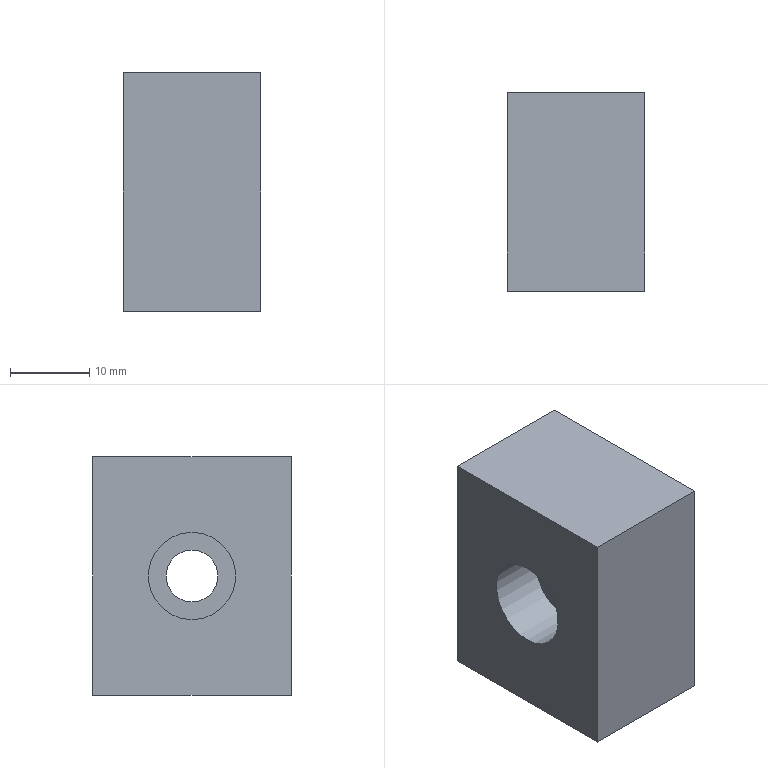Part | STEP file | SPACE-OLATE-INSERT_id702_x_t | 1 solid | 9 faces | box 17.329 x 25 x 30 mm | volume 11989 mm3 | plane 7 | cylinder 2 | commonest cylinder face diameters 6.5 x1 11 x1
STEP:
#1=CARTESIAN_POINT('',(121.671,-163.,93.));
#2=VERTEX_POINT('',#1);
#3=CARTESIAN_POINT('',(121.671,-163.,87.5));
#4=DIRECTION('',(-1.,0.,0.));
#5=DIRECTION('',(0.,0.,1.));
#6=AXIS2_PLACEMENT_3D('',#3,#4,#5);
#7=CIRCLE('',#6,5.5);
#8=EDGE_CURVE('',#2,#2,#7,.T.);
#9=ORIENTED_EDGE('',*,*,#8,.F.);
#10=EDGE_LOOP('',(#9));
#11=FACE_BOUND('',#10,.T.);
#12=CARTESIAN_POINT('',(114.671,-163.,93.));
#13=VERTEX_POINT('',#12);
#14=CARTESIAN_POINT('',(114.671,-163.,87.5));
#15=DIRECTION('',(-1.,0.,0.));
#16=DIRECTION('',(0.,0.,1.));
#17=AXIS2_PLACEMENT_3D('',#14,#15,#16);
#18=CIRCLE('',#17,5.5);
#19=EDGE_CURVE('',#13,#13,#18,.T.);
#20=ORIENTED_EDGE('',*,*,#19,.T.);
#21=EDGE_LOOP('',(#20));
#22=FACE_BOUND('',#21,.T.);
#23=CARTESIAN_POINT('',(114.671,-163.,87.5));
#24=DIRECTION('',(-1.,0.,0.));
#25=DIRECTION('',(0.,0.,1.));
#26=AXIS2_PLACEMENT_3D('',#23,#24,#25);
#27=CYLINDRICAL_SURFACE('',#26,5.5);
#28=ADVANCED_FACE('',(#11,#22),#27,.F.);
#29=ORIENTED_EDGE('',*,*,#19,.F.);
#30=EDGE_LOOP('',(#29));
#31=FACE_BOUND('',#30,.T.);
#32=CARTESIAN_POINT('',(114.671,-175.5,72.5));
#33=VERTEX_POINT('',#32);
#34=CARTESIAN_POINT('',(114.671,-150.5,72.5));
#35=VERTEX_POINT('',#34);
#36=CARTESIAN_POINT('',(114.671,-150.5,72.5));
#37=DIRECTION('',(0.,1.,0.));
#38=VECTOR('',#37,1.);
#39=LINE('',#36,#38);
#40=EDGE_CURVE('',#33,#35,#39,.T.);
#41=ORIENTED_EDGE('',*,*,#40,.F.);
#42=CARTESIAN_POINT('',(114.671,-175.5,102.5));
#43=VERTEX_POINT('',#42);
#44=CARTESIAN_POINT('',(114.671,-175.5,72.5));
#45=DIRECTION('',(0.,0.,-1.));
#46=VECTOR('',#45,1.);
#47=LINE('',#44,#46);
#48=EDGE_CURVE('',#43,#33,#47,.T.);
#49=ORIENTED_EDGE('',*,*,#48,.F.);
#50=CARTESIAN_POINT('',(114.671,-150.5,102.5));
#51=VERTEX_POINT('',#50);
#52=CARTESIAN_POINT('',(114.671,-175.5,102.5));
#53=DIRECTION('',(0.,-1.,0.));
#54=VECTOR('',#53,1.);
#55=LINE('',#52,#54);
#56=EDGE_CURVE('',#51,#43,#55,.T.);
#57=ORIENTED_EDGE('',*,*,#56,.F.);
#58=CARTESIAN_POINT('',(114.671,-150.5,102.5));
#59=DIRECTION('',(0.,0.,1.));
#60=VECTOR('',#59,1.);
#61=LINE('',#58,#60);
#62=EDGE_CURVE('',#35,#51,#61,.T.);
#63=ORIENTED_EDGE('',*,*,#62,.F.);
#64=EDGE_LOOP('',(#41,#49,#57,#63));
#65=FACE_BOUND('',#64,.T.);
#66=CARTESIAN_POINT('',(114.671,-158.476,102.5));
#67=DIRECTION('',(1.,0.,0.));
#68=DIRECTION('',(0.,0.,-1.));
#69=AXIS2_PLACEMENT_3D('',#66,#67,#68);
#70=PLANE('',#69);
#71=ADVANCED_FACE('',(#31,#65),#70,.F.);
#72=CARTESIAN_POINT('',(121.671,-163.,90.75));
#73=VERTEX_POINT('',#72);
#74=CARTESIAN_POINT('',(121.671,-163.,87.5));
#75=DIRECTION('',(1.,0.,0.));
#76=DIRECTION('',(0.,0.,1.));
#77=AXIS2_PLACEMENT_3D('',#74,#75,#76);
#78=CIRCLE('',#77,3.25);
#79=EDGE_CURVE('',#73,#73,#78,.T.);
#80=ORIENTED_EDGE('',*,*,#79,.T.);
#81=EDGE_LOOP('',(#80));
#82=FACE_BOUND('',#81,.T.);
#83=ORIENTED_EDGE('',*,*,#8,.T.);
#84=EDGE_LOOP('',(#83));
#85=FACE_BOUND('',#84,.T.);
#86=CARTESIAN_POINT('',(121.671,-150.5,102.5));
#87=DIRECTION('',(-1.,0.,0.));
#88=DIRECTION('',(0.,0.,1.));
#89=AXIS2_PLACEMENT_3D('',#86,#87,#88);
#90=PLANE('',#89);
#91=ADVANCED_FACE('',(#82,#85),#90,.T.);
#92=CARTESIAN_POINT('',(132.,-175.5,102.5));
#93=VERTEX_POINT('',#92);
#94=CARTESIAN_POINT('',(132.,-175.5,102.5));
#95=DIRECTION('',(-1.,0.,0.));
#96=VECTOR('',#95,1.);
#97=LINE('',#94,#96);
#98=EDGE_CURVE('',#93,#43,#97,.T.);
#99=ORIENTED_EDGE('',*,*,#98,.F.);
#100=CARTESIAN_POINT('',(132.,-150.5,102.5));
#101=VERTEX_POINT('',#100);
#102=CARTESIAN_POINT('',(132.,-120.5,102.5));
#103=DIRECTION('',(0.,1.,0.));
#104=VECTOR('',#103,1.);
#105=LINE('',#102,#104);
#106=EDGE_CURVE('',#93,#101,#105,.T.);
#107=ORIENTED_EDGE('',*,*,#106,.T.);
#108=CARTESIAN_POINT('',(132.,-150.5,102.5));
#109=DIRECTION('',(1.,0.,0.));
#110=VECTOR('',#109,1.);
#111=LINE('',#108,#110);
#112=EDGE_CURVE('',#51,#101,#111,.T.);
#113=ORIENTED_EDGE('',*,*,#112,.F.);
#114=ORIENTED_EDGE('',*,*,#56,.T.);
#115=EDGE_LOOP('',(#99,#107,#113,#114));
#116=FACE_OUTER_BOUND('',#115,.T.);
#117=CARTESIAN_POINT('',(132.,-175.5,102.5));
#118=DIRECTION('',(0.,0.,1.));
#119=DIRECTION('',(1.,0.,0.));
#120=AXIS2_PLACEMENT_3D('',#117,#118,#119);
#121=PLANE('',#120);
#122=ADVANCED_FACE('',(#116),#121,.T.);
#123=ORIENTED_EDGE('',*,*,#112,.T.);
#124=CARTESIAN_POINT('',(132.,-150.5,72.5));
#125=VERTEX_POINT('',#124);
#126=CARTESIAN_POINT('',(132.,-150.5,275.));
#127=DIRECTION('',(0.,0.,-1.));
#128=VECTOR('',#127,1.);
#129=LINE('',#126,#128);
#130=EDGE_CURVE('',#101,#125,#129,.T.);
#131=ORIENTED_EDGE('',*,*,#130,.T.);
#132=CARTESIAN_POINT('',(132.,-150.5,72.5));
#133=DIRECTION('',(1.,0.,0.));
#134=VECTOR('',#133,1.);
#135=LINE('',#132,#134);
#136=EDGE_CURVE('',#35,#125,#135,.T.);
#137=ORIENTED_EDGE('',*,*,#136,.F.);
#138=ORIENTED_EDGE('',*,*,#62,.T.);
#139=EDGE_LOOP('',(#123,#131,#137,#138));
#140=FACE_OUTER_BOUND('',#139,.T.);
#141=CARTESIAN_POINT('',(132.,-150.5,102.5));
#142=DIRECTION('',(0.,1.,0.));
#143=DIRECTION('',(0.,0.,1.));
#144=AXIS2_PLACEMENT_3D('',#141,#142,#143);
#145=PLANE('',#144);
#146=ADVANCED_FACE('',(#140),#145,.T.);
#147=ORIENTED_EDGE('',*,*,#136,.T.);
#148=CARTESIAN_POINT('',(132.,-175.5,72.5));
#149=VERTEX_POINT('',#148);
#150=CARTESIAN_POINT('',(132.,-120.5,72.5));
#151=DIRECTION('',(0.,-1.,0.));
#152=VECTOR('',#151,1.);
#153=LINE('',#150,#152);
#154=EDGE_CURVE('',#125,#149,#153,.T.);
#155=ORIENTED_EDGE('',*,*,#154,.T.);
#156=CARTESIAN_POINT('',(132.,-175.5,72.5));
#157=DIRECTION('',(1.,0.,0.));
#158=VECTOR('',#157,1.);
#159=LINE('',#156,#158);
#160=EDGE_CURVE('',#33,#149,#159,.T.);
#161=ORIENTED_EDGE('',*,*,#160,.F.);
#162=ORIENTED_EDGE('',*,*,#40,.T.);
#163=EDGE_LOOP('',(#147,#155,#161,#162));
#164=FACE_OUTER_BOUND('',#163,.T.);
#165=CARTESIAN_POINT('',(132.,-150.5,72.5));
#166=DIRECTION('',(0.,0.,-1.));
#167=DIRECTION('',(-1.,0.,0.));
#168=AXIS2_PLACEMENT_3D('',#165,#166,#167);
#169=PLANE('',#168);
#170=ADVANCED_FACE('',(#164),#169,.T.);
#171=ORIENTED_EDGE('',*,*,#160,.T.);
#172=CARTESIAN_POINT('',(132.,-175.5,275.));
#173=DIRECTION('',(0.,0.,1.));
#174=VECTOR('',#173,1.);
#175=LINE('',#172,#174);
#176=EDGE_CURVE('',#149,#93,#175,.T.);
#177=ORIENTED_EDGE('',*,*,#176,.T.);
#178=ORIENTED_EDGE('',*,*,#98,.T.);
#179=ORIENTED_EDGE('',*,*,#48,.T.);
#180=EDGE_LOOP('',(#171,#177,#178,#179));
#181=FACE_OUTER_BOUND('',#180,.T.);
#182=CARTESIAN_POINT('',(132.,-175.5,72.5));
#183=DIRECTION('',(0.,-1.,0.));
#184=DIRECTION('',(0.,0.,-1.));
#185=AXIS2_PLACEMENT_3D('',#182,#183,#184);
#186=PLANE('',#185);
#187=ADVANCED_FACE('',(#181),#186,.T.);
#188=CARTESIAN_POINT('',(132.,-163.,90.75));
#189=VERTEX_POINT('',#188);
#190=CARTESIAN_POINT('',(132.,-163.,87.5));
#191=DIRECTION('',(1.,0.,0.));
#192=DIRECTION('',(0.,0.,1.));
#193=AXIS2_PLACEMENT_3D('',#190,#191,#192);
#194=CIRCLE('',#193,3.25);
#195=EDGE_CURVE('',#189,#189,#194,.T.);
#196=ORIENTED_EDGE('',*,*,#195,.T.);
#197=EDGE_LOOP('',(#196));
#198=FACE_BOUND('',#197,.T.);
#199=ORIENTED_EDGE('',*,*,#79,.F.);
#200=EDGE_LOOP('',(#199));
#201=FACE_BOUND('',#200,.T.);
#202=CARTESIAN_POINT('',(132.,-163.,87.5));
#203=DIRECTION('',(-1.,0.,0.));
#204=DIRECTION('',(0.,0.,1.));
#205=AXIS2_PLACEMENT_3D('',#202,#203,#204);
#206=CYLINDRICAL_SURFACE('',#205,3.25);
#207=ADVANCED_FACE('',(#198,#201),#206,.F.);
#208=ORIENTED_EDGE('',*,*,#195,.F.);
#209=EDGE_LOOP('',(#208));
#210=FACE_BOUND('',#209,.T.);
#211=ORIENTED_EDGE('',*,*,#154,.F.);
#212=ORIENTED_EDGE('',*,*,#130,.F.);
#213=ORIENTED_EDGE('',*,*,#106,.F.);
#214=ORIENTED_EDGE('',*,*,#176,.F.);
#215=EDGE_LOOP('',(#211,#212,#213,#214));
#216=FACE_BOUND('',#215,.T.);
#217=CARTESIAN_POINT('',(132.,-120.5,275.));
#218=DIRECTION('',(-1.,0.,0.));
#219=DIRECTION('',(0.,0.,1.));
#220=AXIS2_PLACEMENT_3D('',#217,#218,#219);
#221=PLANE('',#220);
#222=ADVANCED_FACE('',(#210,#216),#221,.F.);
#223=CLOSED_SHELL('',(#28,#71,#91,#122,#146,#170,#187,#207,#222));
#224=MANIFOLD_SOLID_BREP('',#223);
#225=(LENGTH_UNIT()NAMED_UNIT(*)SI_UNIT(.MILLI.,.METRE.));
#226=UNCERTAINTY_MEASURE_WITH_UNIT(LENGTH_MEASURE(0.00002),#225,'','');
#227=(NAMED_UNIT(*)PLANE_ANGLE_UNIT()SI_UNIT($,.RADIAN.));
#228=PLANE_ANGLE_MEASURE_WITH_UNIT(PLANE_ANGLE_MEASURE(0.01745),#227);
#229=DIMENSIONAL_EXPONENTS(0.,0.,0.,0.,0.,0.,0.);
#230=(CONVERSION_BASED_UNIT('DEGREE',#228)NAMED_UNIT(#229)PLANE_ANGLE_UNIT());
#231=(NAMED_UNIT(*)SI_UNIT($,.STERADIAN.)SOLID_ANGLE_UNIT());
#232=(GEOMETRIC_REPRESENTATION_CONTEXT(3)GLOBAL_UNCERTAINTY_ASSIGNED_CONTEXT((#226))GLOBAL_UNIT_ASSIGNED_CONTEXT((#225,#230,#231))REPRESENTATION_CONTEXT('',''));
#233=ADVANCED_BREP_SHAPE_REPRESENTATION('',(#224),#232);